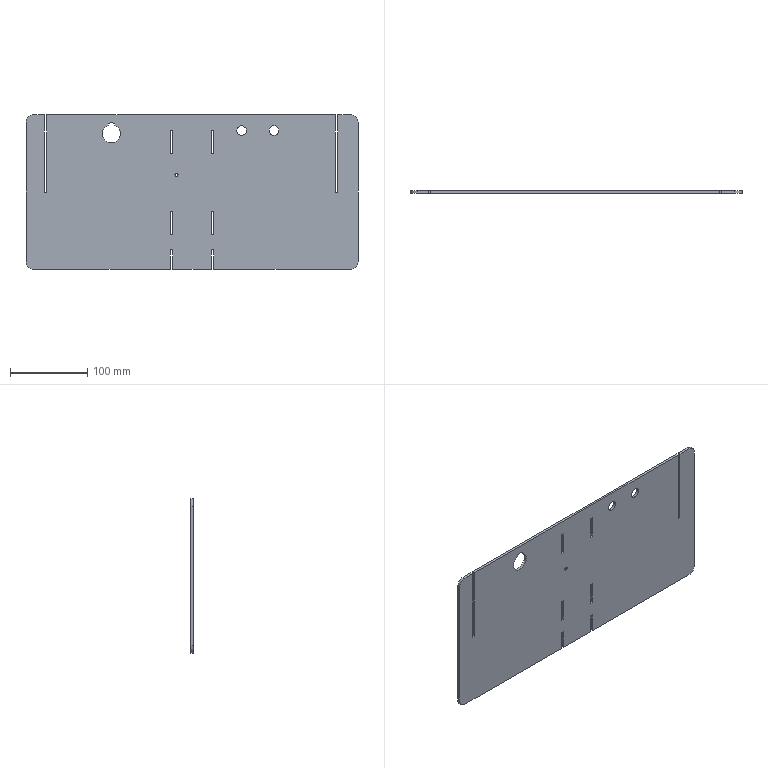Part | SolidWorks | features FlatPattern 1, SMBaseFlange 1, SheetMetal 1 | 1 solid | 53 faces | box 430 x 3.2 x 200 mm | volume 268842 mm3 | plane 40 | cylinder 13 | commonest cylinder face diameters 12.5 x4 20 x4 4 x2 28 x2 23.5 x1